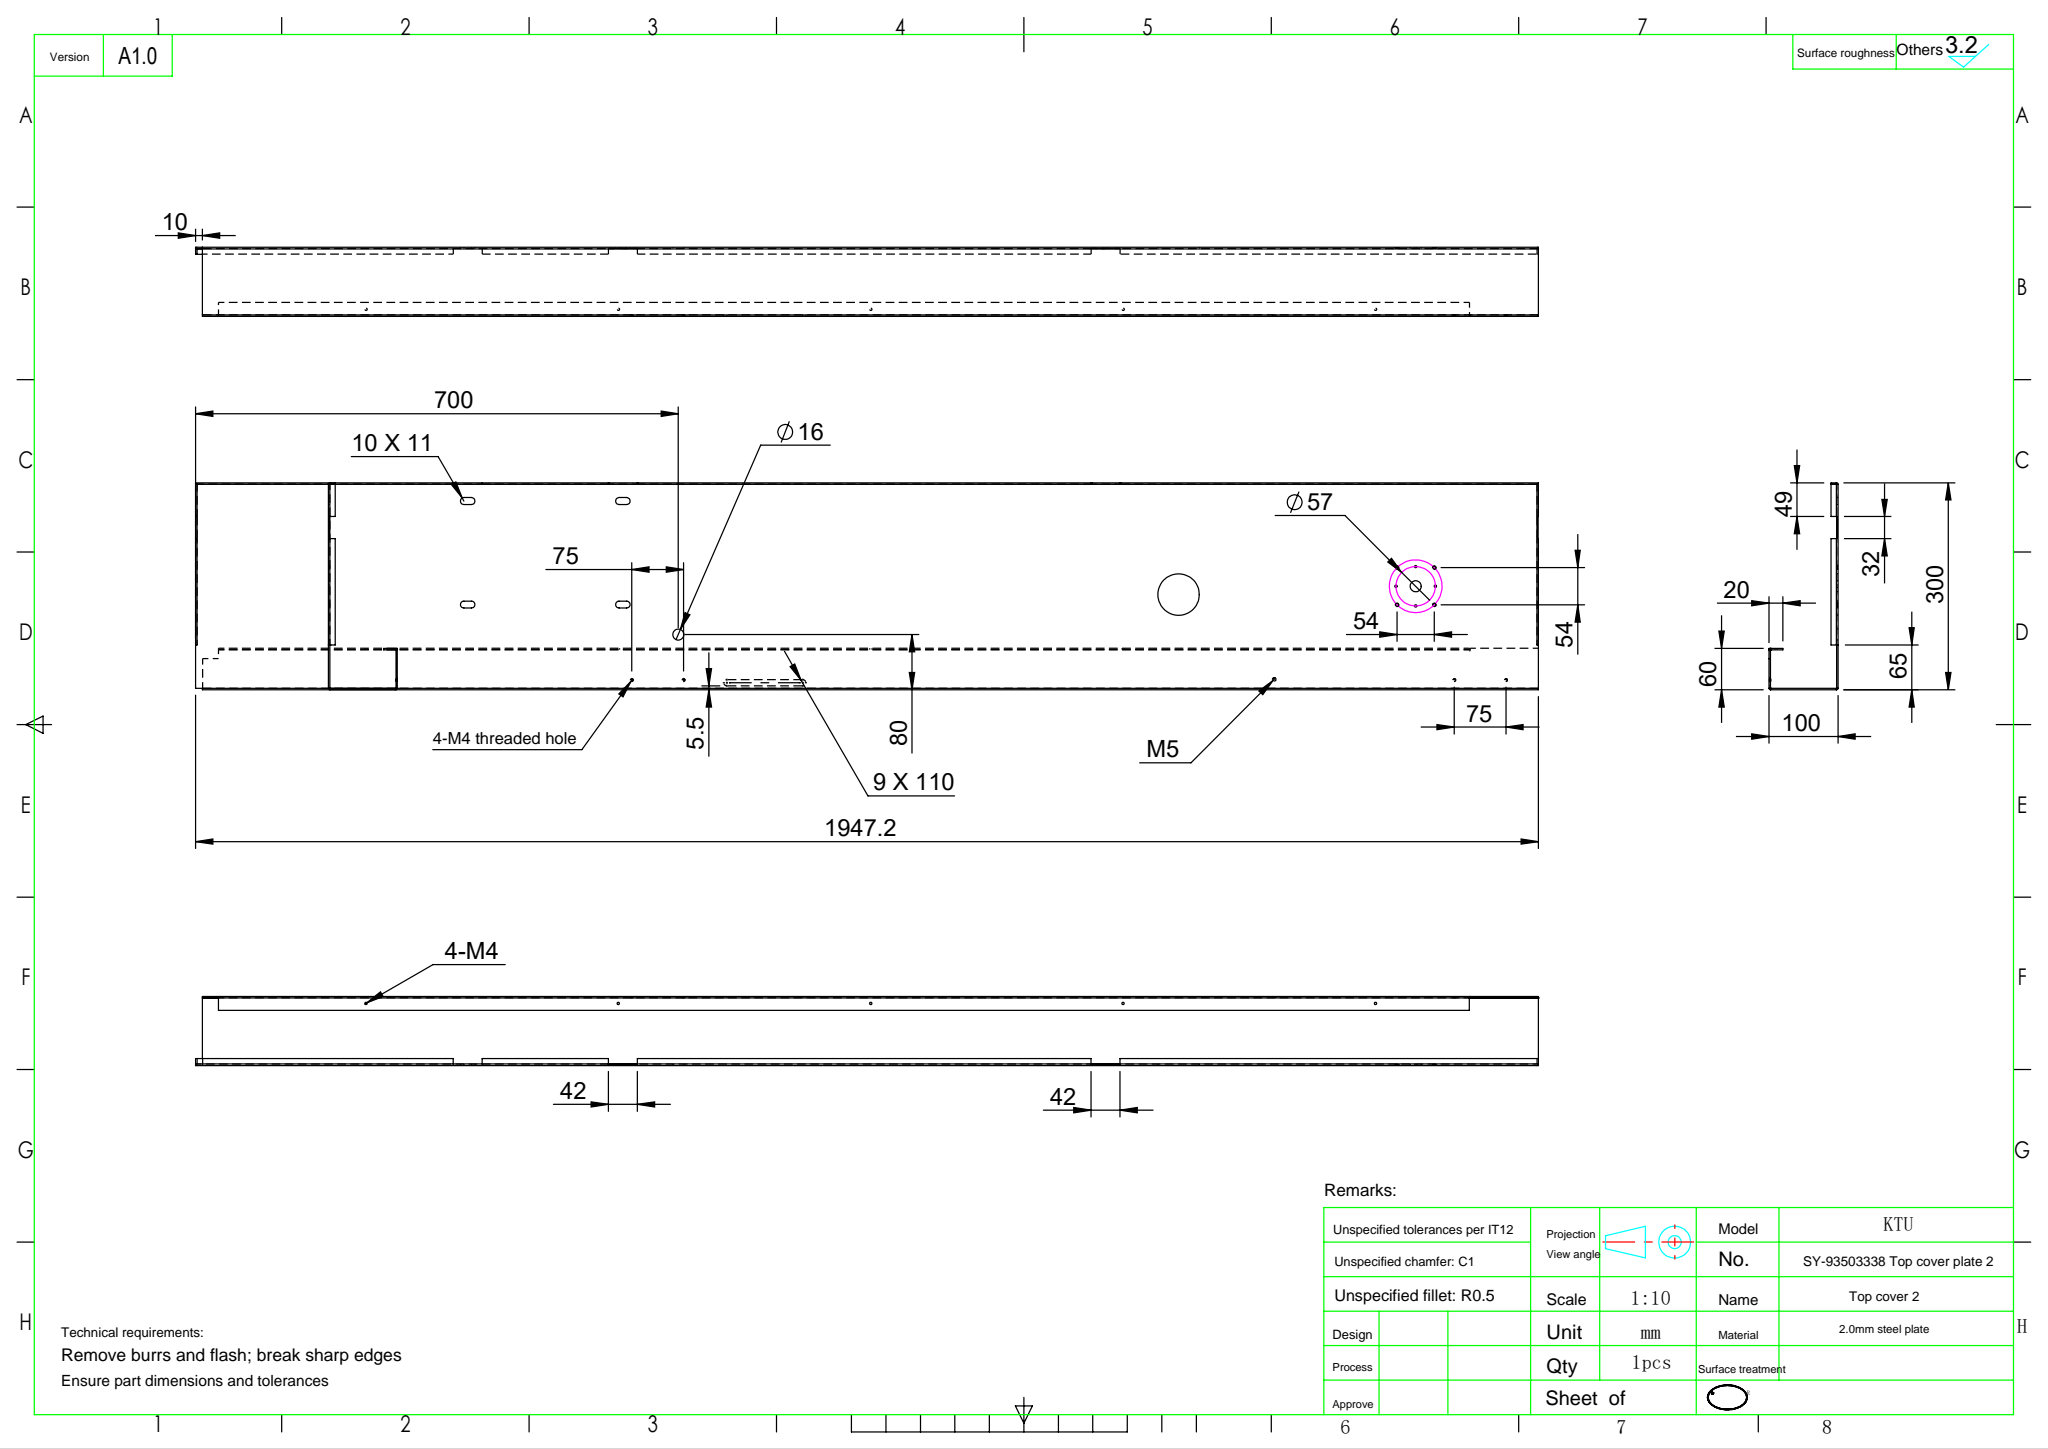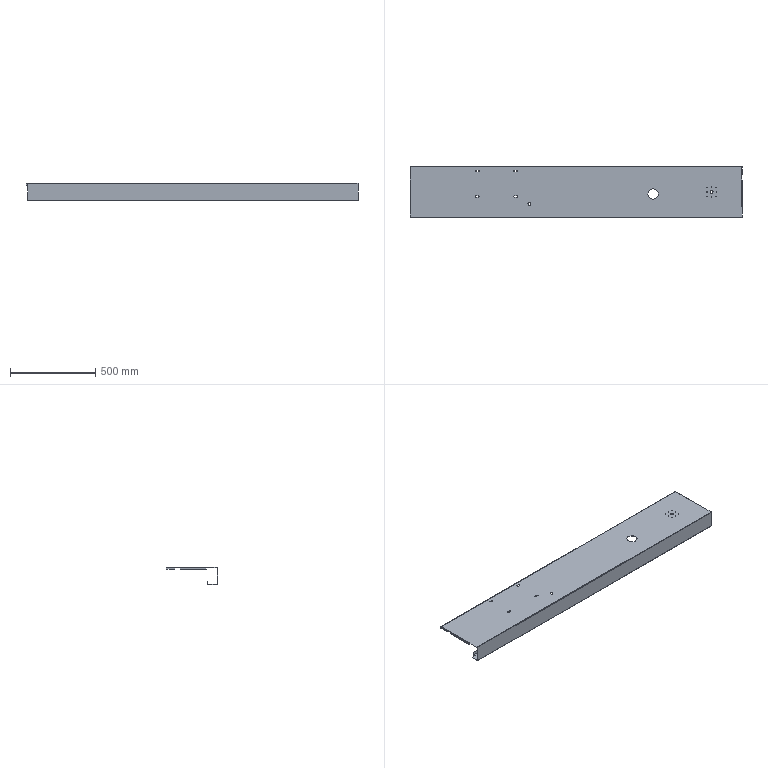Part | SolidWorks | features Cut 8, EdgeFlange 5, HoleWzd 3, ICE 3, 3DProfileFeature 1, CirPattern 1, FlatPattern 1, LPattern 1, MirrorPattern 1, SMBaseFlange 1, SheetMetal 1 | 1 solid | 178 faces | box 1947 x 300 x 100 mm | volume 1854038 mm3 | plane 100 | cylinder 70 | cone 8 | commonest cylinder face diameters 3.3 x26 10 x12 4.2 x10 0.4 x6 4.4 x6 16 x4